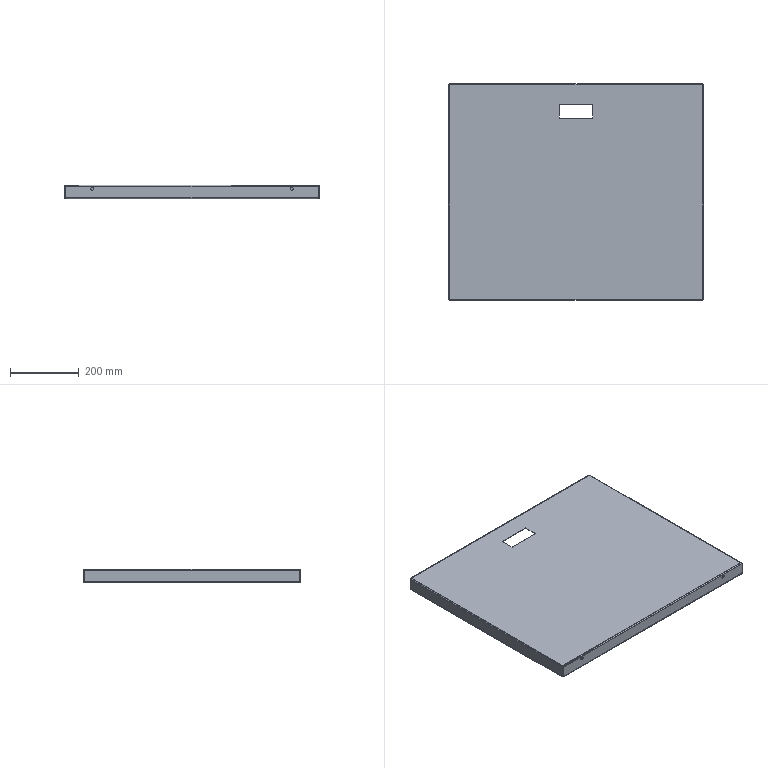Part | SolidWorks | features EdgeFlange 2, FlatPattern 1, HoleWzd 1, SMBaseFlange 1, SheetMetal 1 | 1 solid | 78 faces | box 740 x 630 x 40 mm | volume 914335 mm3 | plane 42 | cylinder 20 | spline 16 | commonest cylinder face diameters 4 x8 7 x8 9 x4